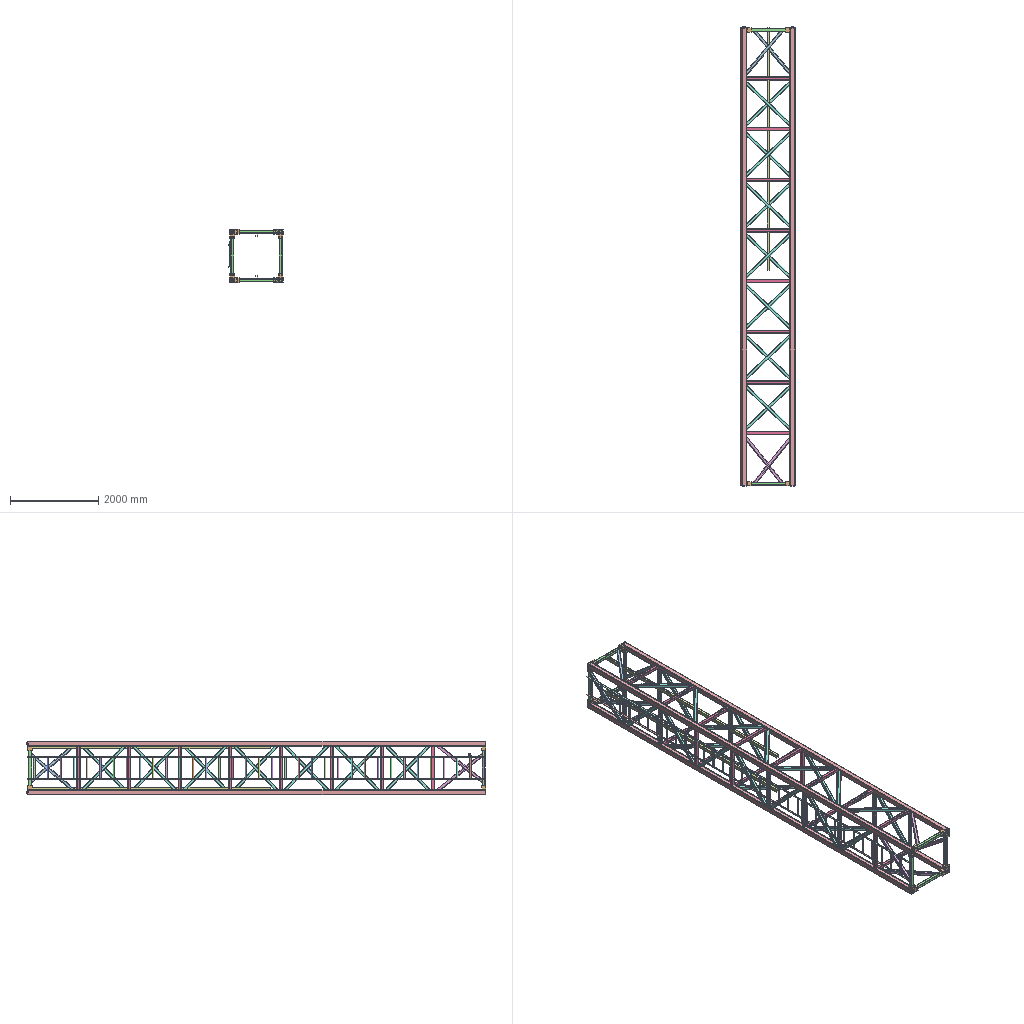Assembly | SolidWorks | 13 different items | 115 placed | box 1235 x 10440 x 1220 mm
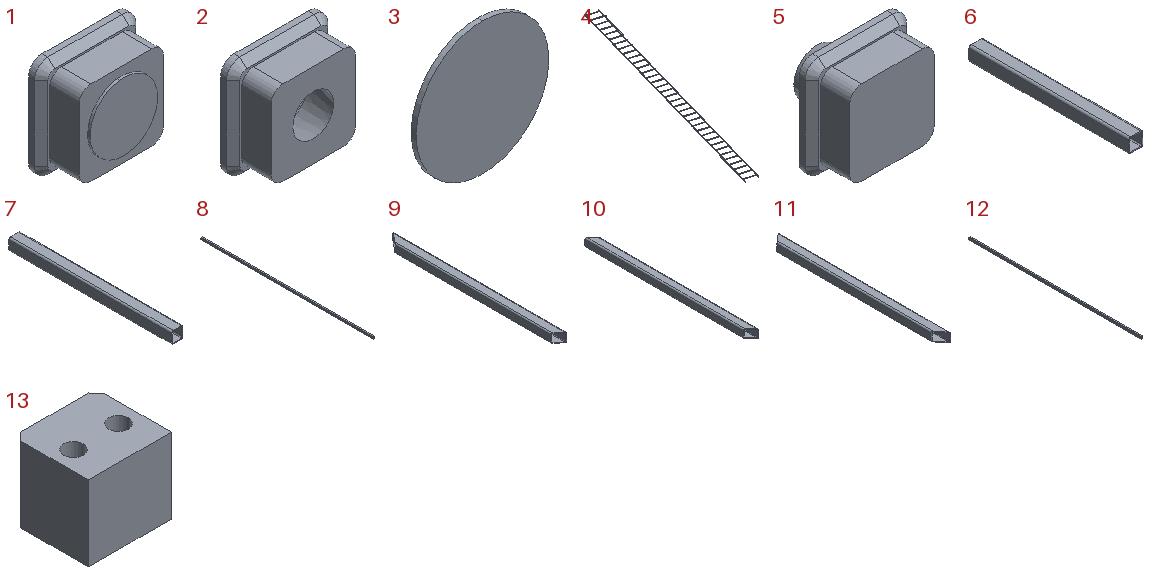Parts list (item | name | quantity | parent item | size | volume | features):
1 | (subassembly) | x4 | - | 120 x 53 x 120 mm | 407856 mm3 | -
2 | - | x4 | in 1 | 120 x 50 x 120 mm | 392776 mm3 | features Chamfer 1, Extrusion 1, ICE 1, RevCut 1
3 | - | x4 | in 1 | 80 x 3 x 80 mm | 15080 mm3 | features Extrusion 1
4 | - | x1 | - | 3347 x 10135 x 40 mm | 8856041 mm3 | features WeldMemberFeat 2, Chamfer 1, LPattern 1, Sweep 1, WeldCornerFeat 1, WeldmentFeature 1
5 | - | x4 | - | 120 x 90 x 120 mm | 672208 mm3 | features Chamfer 2, ICE 2, Revolution 1
6 | - | x8 | - | 70 x 780 x 70 mm | 963783 mm3 | features WeldMemberFeat 1, WeldmentFeature 1
7 | - | x32 | - | 70 x 980 x 70 mm | 1210907 mm3 | features WeldMemberFeat 1, WeldmentFeature 1
8 | - | x4 | - | 120 x 10370 x 120 mm | 43669629 mm3 | features WeldMemberFeat 1, WeldmentFeature 1
9 | - | x4 | - | 70 x 1340 x 70 mm | 1567074 mm3 | features ICE 1, WeldMemberFeat 1, WeldmentFeature 1
10 | - | x28 | - | 70 x 1421 x 70 mm | 1672765 mm3 | features ICE 1, WeldMemberFeat 1, WeldmentFeature 1
11 | - | x4 | - | 70 x 1302 x 70 mm | 1520953 mm3 | features ICE 1, WeldMemberFeat 1, WeldmentFeature 1
12 | - | x2 | - | 60 x 5500 x 80 mm | 6795907 mm3 | features WeldMemberFeat 1, WeldmentFeature 1
13 | - | x16 | - | 110 x 100 x 100 mm | 983814 mm3 | features Chamfer 1, Extrusion 1, HoleWzd 1
Mates (type | each side: item.copy, entity, surface, feature):
In the top assembly
Symmetric | 8.1 face plane Cold-formed Hollow Structural Square Steel(gb t6728-2002) 120×120×10(1) | 8.2 face plane Cold-formed Hollow Structural Square Steel(gb t6728-2002) 120×120×10(1) | assembly plane
DistanceDim | assembly plane | 8.1 face plane Cold-formed Hollow Structural Square Steel(gb t6728-2002) 120×120×10(1)
Coincident | 8.3 face plane Cold-formed Hollow Structural Square Steel(gb t6728-2002) 120×120×10(1) | assembly plane
Coincident | 8.1 face plane Cold-formed Hollow Structural Square Steel(gb t6728-2002) 120×120×10(1) | 2.1 face plane Boss-Extrude1
Width | 2.1 face plane Boss-Extrude2 | 2.1 face plane Boss-Extrude2 | 8.1 face plane Cold-formed Hollow Structural Square Steel(gb t6728-2002) 120×120×10(1) | 8.1 face plane Cold-formed Hollow Structural Square Steel(gb t6728-2002) 120×120×10(1)
Width | 8.1 face plane Cold-formed Hollow Structural Square Steel(gb t6728-2002) 120×120×10(1) | 8.1 face plane Cold-formed Hollow Structural Square Steel(gb t6728-2002) 120×120×10(1) | 2.1 face plane Boss-Extrude1 | 2.1 face plane Boss-Extrude1
Coincident | 8.1 face plane Cold-formed Hollow Structural Square Steel(gb t6728-2002) 120×120×10(1) | 5.1 face plane Boss-Extrude1
Width | 8.1 face plane Cold-formed Hollow Structural Square Steel(gb t6728-2002) 120×120×10(1) | 8.1 face plane Cold-formed Hollow Structural Square Steel(gb t6728-2002) 120×120×10(1) | 5.1 face plane Boss-Extrude1 | 5.1 face plane Boss-Extrude1 | 2 times
Coincident | 13.1 face plane Boss-Extrude1 | 2.2 face plane Boss-Extrude1
Width | 13.1 face plane Boss-Extrude1 | 13.1 face plane Boss-Extrude1 | 8.3 face plane Cold-formed Hollow Structural Square Steel(gb t6728-2002) 120×120×10(1) | 8.3 face plane Cold-formed Hollow Structural Square Steel(gb t6728-2002) 120×120×10(1)
Coincident | 13.1 face plane Boss-Extrude1 | 8.3 face plane Cold-formed Hollow Structural Square Steel(gb t6728-2002) 120×120×10(1)
Coincident | 8.3 face plane Cold-formed Hollow Structural Square Steel(gb t6728-2002) 120×120×10(1) | 13.2 face plane Boss-Extrude1
Coincident | 13.1 face plane Boss-Extrude1 | 13.2 face plane Boss-Extrude1
Width | 13.2 face plane Boss-Extrude1 | 13.2 face plane Boss-Extrude1 | 8.3 face plane Cold-formed Hollow Structural Square Steel(gb t6728-2002) 120×120×10(1) | 8.3 face plane Cold-formed Hollow Structural Square Steel(gb t6728-2002) 120×120×10(1)
Coincident | 13.3 face plane Boss-Extrude1 | 13.4 face plane Boss-Extrude1
Coincident | 13.1 face plane Boss-Extrude1 | 13.4 face plane Boss-Extrude1 | 2 times
Coincident | 13.2 face plane Boss-Extrude1 | 13.3 face plane Boss-Extrude1 | 2 times
Coincident | 5.2 face plane Boss-Extrude1 | 13.3 face plane Boss-Extrude1
Coincident | 6.1 face plane feature 19 (WeldMemberFeat) (+4 more in 5 files) Cold-formed Hollow Structural Square Steel(gb t6728-2002) 70×70×5(1) | 6.2 face plane feature 19 (WeldMemberFeat) (+4 more in 5 files) Cold-formed Hollow Structural Square Steel(gb t6728-2002) 70×70×5(1) | 2 times
Width | 6.2 face plane feature 19 (WeldMemberFeat) (+4 more in 5 files) Cold-formed Hollow Structural Square Steel(gb t6728-2002) 70×70×5(1) | 6.2 face plane feature 19 (WeldMemberFeat) (+4 more in 5 files) Cold-formed Hollow Structural Square Steel(gb t6728-2002) 70×70×5(1) | 13.5 face plane Boss-Extrude1 | 13.5 face plane Boss-Extrude1
Coincident | 13.1 face plane Boss-Extrude1 | 6.1 face plane feature 19 (WeldMemberFeat) (+4 more in 5 files) Cold-formed Hollow Structural Square Steel(gb t6728-2002) 70×70×5(1)
Width | 6.1 face plane feature 19 (WeldMemberFeat) (+4 more in 5 files) Cold-formed Hollow Structural Square Steel(gb t6728-2002) 70×70×5(1) | 6.1 face plane feature 19 (WeldMemberFeat) (+4 more in 5 files) Cold-formed Hollow Structural Square Steel(gb t6728-2002) 70×70×5(1) | 13.1 face plane Boss-Extrude1 | 13.1 face plane Boss-Extrude1
Width | 13.1 face plane Boss-Extrude1 | 13.1 face plane Boss-Extrude1 | 6.1 face plane feature 19 (WeldMemberFeat) (+4 more in 5 files) Cold-formed Hollow Structural Square Steel(gb t6728-2002) 70×70×5(1) | 6.1 face plane feature 19 (WeldMemberFeat) (+4 more in 5 files) Cold-formed Hollow Structural Square Steel(gb t6728-2002) 70×70×5(1)
Coincident | 6.3 face plane feature 19 (WeldMemberFeat) (+4 more in 5 files) Cold-formed Hollow Structural Square Steel(gb t6728-2002) 70×70×5(1) | 6.4 face plane feature 19 (WeldMemberFeat) (+4 more in 5 files) Cold-formed Hollow Structural Square Steel(gb t6728-2002) 70×70×5(1) | 2 times
Coincident | 13.2 face plane Boss-Extrude1 | 6.3 face plane feature 19 (WeldMemberFeat) (+4 more in 5 files) Cold-formed Hollow Structural Square Steel(gb t6728-2002) 70×70×5(1)
Width | 6.3 face plane feature 19 (WeldMemberFeat) (+4 more in 5 files) Cold-formed Hollow Structural Square Steel(gb t6728-2002) 70×70×5(1) | 6.3 face plane feature 19 (WeldMemberFeat) (+4 more in 5 files) Cold-formed Hollow Structural Square Steel(gb t6728-2002) 70×70×5(1) | 13.2 face plane Boss-Extrude1 | 13.2 face plane Boss-Extrude1 | 2 times
Width | 6.4 face plane feature 19 (WeldMemberFeat) (+4 more in 5 files) Cold-formed Hollow Structural Square Steel(gb t6728-2002) 70×70×5(1) | 6.4 face plane feature 19 (WeldMemberFeat) (+4 more in 5 files) Cold-formed Hollow Structural Square Steel(gb t6728-2002) 70×70×5(1) | 13.3 face plane Boss-Extrude1 | 13.3 face plane Boss-Extrude1
Width | 7.1 face plane feature 19 (WeldMemberFeat) (+4 more in 5 files) Cold-formed Hollow Structural Square Steel(gb t6728-2002) 70×70×5(1) | 7.1 face plane feature 19 (WeldMemberFeat) (+4 more in 5 files) Cold-formed Hollow Structural Square Steel(gb t6728-2002) 70×70×5(1) | 8.4 face plane Cold-formed Hollow Structural Square Steel(gb t6728-2002) 120×120×10(1) | 8.4 face plane Cold-formed Hollow Structural Square Steel(gb t6728-2002) 120×120×10(1)
Coincident | 7.1 face plane feature 19 (WeldMemberFeat) (+4 more in 5 files) Cold-formed Hollow Structural Square Steel(gb t6728-2002) 70×70×5(1) | 8.4 face plane Cold-formed Hollow Structural Square Steel(gb t6728-2002) 120×120×10(1)
DistanceDim | 2.2 face plane Boss-Extrude1 | 7.1 face plane feature 19 (WeldMemberFeat) (+4 more in 5 files) Cold-formed Hollow Structural Square Steel(gb t6728-2002) 70×70×5(1)
Coincident | 10.1 face plane Cut-Extrude1 | 8.4 face plane Cold-formed Hollow Structural Square Steel(gb t6728-2002) 120×120×10(1)
Coincident | 8.3 face plane Cold-formed Hollow Structural Square Steel(gb t6728-2002) 120×120×10(1) | 10.2 face plane Cut-Extrude1
Coincident | 10.1 face plane feature 19 (WeldMemberFeat) (+4 more in 5 files) Cold-formed Hollow Structural Square Steel(gb t6728-2002) 70×70×5(1) | 10.2 face plane feature 19 (WeldMemberFeat) (+4 more in 5 files) Cold-formed Hollow Structural Square Steel(gb t6728-2002) 70×70×5(1)
DistanceDim | 10.2 edge | 7.2 face plane feature 19 (WeldMemberFeat) (+4 more in 5 files) Cold-formed Hollow Structural Square Steel(gb t6728-2002) 70×70×5(1)
Coincident | 8.1 face plane Cold-formed Hollow Structural Square Steel(gb t6728-2002) 120×120×10(1) | 10.3 face plane Cut-Extrude1
Coincident | 7.3 face plane feature 19 (WeldMemberFeat) (+4 more in 5 files) Cold-formed Hollow Structural Square Steel(gb t6728-2002) 70×70×5(1) | 10.3 face plane feature 19 (WeldMemberFeat) (+4 more in 5 files) Cold-formed Hollow Structural Square Steel(gb t6728-2002) 70×70×5(1)
DistanceDim | 10.3 edge | 7.3 face plane feature 19 (WeldMemberFeat) (+4 more in 5 files) Cold-formed Hollow Structural Square Steel(gb t6728-2002) 70×70×5(1)
Coincident | 10.3 face plane feature 19 (WeldMemberFeat) (+4 more in 5 files) Cold-formed Hollow Structural Square Steel(gb t6728-2002) 70×70×5(1) | 10.4 face plane feature 19 (WeldMemberFeat) (+4 more in 5 files) Cold-formed Hollow Structural Square Steel(gb t6728-2002) 70×70×5(1)
Coincident | 8.2 face plane Cold-formed Hollow Structural Square Steel(gb t6728-2002) 120×120×10(1) | 10.4 face plane Cut-Extrude1
DistanceDim | 10.4 edge | 7.4 face plane feature 19 (WeldMemberFeat) (+4 more in 5 files) Cold-formed Hollow Structural Square Steel(gb t6728-2002) 70×70×5(1)
Coincident | 6.2 face plane feature 19 (WeldMemberFeat) (+4 more in 5 files) Cold-formed Hollow Structural Square Steel(gb t6728-2002) 70×70×5(1) | 11.1 face plane Cut-Extrude1
Coincident | 6.2 face plane feature 19 (WeldMemberFeat) (+4 more in 5 files) Cold-formed Hollow Structural Square Steel(gb t6728-2002) 70×70×5(1) | 11.1 face plane feature 19 (WeldMemberFeat) (+4 more in 5 files) Cold-formed Hollow Structural Square Steel(gb t6728-2002) 70×70×5(1)
Coincident | 8.3 face plane Cold-formed Hollow Structural Square Steel(gb t6728-2002) 120×120×10(1) | 11.1 face plane Cut-Extrude1
Coincident | 8.2 face plane Cold-formed Hollow Structural Square Steel(gb t6728-2002) 120×120×10(1) | 11.2 face plane Cut-Extrude1
Coincident | 7.5 face plane feature 19 (WeldMemberFeat) (+4 more in 5 files) Cold-formed Hollow Structural Square Steel(gb t6728-2002) 70×70×5(1) | 11.2 face plane feature 19 (WeldMemberFeat) (+4 more in 5 files) Cold-formed Hollow Structural Square Steel(gb t6728-2002) 70×70×5(1)
Coincident | 6.5 face plane feature 19 (WeldMemberFeat) (+4 more in 5 files) Cold-formed Hollow Structural Square Steel(gb t6728-2002) 70×70×5(1) | 11.2 face plane Cut-Extrude1
Coincident | 7.1 face plane feature 19 (WeldMemberFeat) (+4 more in 5 files) Cold-formed Hollow Structural Square Steel(gb t6728-2002) 70×70×5(1) | 7.6 face plane feature 19 (WeldMemberFeat) (+4 more in 5 files) Cold-formed Hollow Structural Square Steel(gb t6728-2002) 70×70×5(1)
Coincident | 8.3 face plane Cold-formed Hollow Structural Square Steel(gb t6728-2002) 120×120×10(1) | 7.6 face plane feature 19 (WeldMemberFeat) (+4 more in 5 files) Cold-formed Hollow Structural Square Steel(gb t6728-2002) 70×70×5(1)
Width | 7.6 face plane feature 19 (WeldMemberFeat) (+4 more in 5 files) Cold-formed Hollow Structural Square Steel(gb t6728-2002) 70×70×5(1) | 7.6 face plane feature 19 (WeldMemberFeat) (+4 more in 5 files) Cold-formed Hollow Structural Square Steel(gb t6728-2002) 70×70×5(1) | 8.3 face plane Cold-formed Hollow Structural Square Steel(gb t6728-2002) 120×120×10(1) | 8.3 face plane Cold-formed Hollow Structural Square Steel(gb t6728-2002) 120×120×10(1)
Coincident | 7.6 face plane feature 19 (WeldMemberFeat) (+4 more in 5 files) Cold-formed Hollow Structural Square Steel(gb t6728-2002) 70×70×5(1) | 7.7 face plane feature 19 (WeldMemberFeat) (+4 more in 5 files) Cold-formed Hollow Structural Square Steel(gb t6728-2002) 70×70×5(1) | 2 times
Width | 7.7 face plane feature 19 (WeldMemberFeat) (+4 more in 5 files) Cold-formed Hollow Structural Square Steel(gb t6728-2002) 70×70×5(1) | 7.7 face plane feature 19 (WeldMemberFeat) (+4 more in 5 files) Cold-formed Hollow Structural Square Steel(gb t6728-2002) 70×70×5(1) | 8.2 face plane Cold-formed Hollow Structural Square Steel(gb t6728-2002) 120×120×10(1) | 8.2 face plane Cold-formed Hollow Structural Square Steel(gb t6728-2002) 120×120×10(1)
Coincident | 4.1 face plane Gb/t 704—1988Hot-rolled Flat Steel 40×6(1) | 6.4 face plane feature 19 (WeldMemberFeat) (+4 more in 5 files) Cold-formed Hollow Structural Square Steel(gb t6728-2002) 70×70×5(1)
Width | 8.3 face plane Cold-formed Hollow Structural Square Steel(gb t6728-2002) 120×120×10(1) | 8.1 face plane Cold-formed Hollow Structural Square Steel(gb t6728-2002) 120×120×10(1) | 4.1 face plane Gb/t 704—1988Hot-rolled Flat Steel 40×6(1) | 4.1 face plane Gb/t 704—1988Hot-rolled Flat Steel 40×6(1)
Coincident | 4.1 face plane Gb/t 704—1988Hot-rolled Flat Steel 40×6(1) | 2.2 face plane Boss-Extrude1
Coincident | 6.2 face plane feature 19 (WeldMemberFeat) (+4 more in 5 files) Cold-formed Hollow Structural Square Steel(gb t6728-2002) 70×70×5(1) | 12.1 face plane Cold-formed Hollow Structural Rectangular Steel(gb t6728-2002) 80×60×5(1)
Coincident | 12.1 plane | assembly plane
Coincident | 12.1 face plane Cold-formed Hollow Structural Rectangular Steel(gb t6728-2002) 80×60×5(1) | 13.5 face plane Boss-Extrude1
Coincident | 9.1 face plane Cut-Extrude1 | 6.1 face plane feature 19 (WeldMemberFeat) (+4 more in 5 files) Cold-formed Hollow Structural Square Steel(gb t6728-2002) 70×70×5(1)
Coincident | 9.1 face plane feature 19 (WeldMemberFeat) (+4 more in 5 files) Cold-formed Hollow Structural Square Steel(gb t6728-2002) 70×70×5(1) | 6.1 face plane feature 19 (WeldMemberFeat) (+4 more in 5 files) Cold-formed Hollow Structural Square Steel(gb t6728-2002) 70×70×5(1)
Coincident | 9.1 face plane Cut-Extrude1 | 8.4 face plane Cold-formed Hollow Structural Square Steel(gb t6728-2002) 120×120×10(1)
Coincident | 6.6 face plane feature 19 (WeldMemberFeat) (+4 more in 5 files) Cold-formed Hollow Structural Square Steel(gb t6728-2002) 70×70×5(1) | 9.2 face plane Cut-Extrude1
Coincident | 6.6 face plane feature 19 (WeldMemberFeat) (+4 more in 5 files) Cold-formed Hollow Structural Square Steel(gb t6728-2002) 70×70×5(1) | 9.2 face plane feature 19 (WeldMemberFeat) (+4 more in 5 files) Cold-formed Hollow Structural Square Steel(gb t6728-2002) 70×70×5(1)
Coincident | 8.1 face plane Cold-formed Hollow Structural Square Steel(gb t6728-2002) 120×120×10(1) | 9.2 face plane Cut-Extrude1
Coincident | 6.3 face plane feature 19 (WeldMemberFeat) (+4 more in 5 files) Cold-formed Hollow Structural Square Steel(gb t6728-2002) 70×70×5(1) | 9.3 face plane Cut-Extrude1
Coincident | 6.3 face plane feature 19 (WeldMemberFeat) (+4 more in 5 files) Cold-formed Hollow Structural Square Steel(gb t6728-2002) 70×70×5(1) | 9.3 face plane feature 19 (WeldMemberFeat) (+4 more in 5 files) Cold-formed Hollow Structural Square Steel(gb t6728-2002) 70×70×5(1)
Coincident | 8.3 face plane Cold-formed Hollow Structural Square Steel(gb t6728-2002) 120×120×10(1) | 9.3 face plane Cut-Extrude1
Coincident | 6.7 face plane feature 19 (WeldMemberFeat) (+4 more in 5 files) Cold-formed Hollow Structural Square Steel(gb t6728-2002) 70×70×5(1) | 9.4 face plane Cut-Extrude1
Coincident | 6.7 face plane feature 19 (WeldMemberFeat) (+4 more in 5 files) Cold-formed Hollow Structural Square Steel(gb t6728-2002) 70×70×5(1) | 9.4 face plane feature 19 (WeldMemberFeat) (+4 more in 5 files) Cold-formed Hollow Structural Square Steel(gb t6728-2002) 70×70×5(1)
Coincident | 8.2 face plane Cold-formed Hollow Structural Square Steel(gb t6728-2002) 120×120×10(1) | 9.4 face plane Cut-Extrude1
Coincident | 8.1 face plane Cold-formed Hollow Structural Square Steel(gb t6728-2002) 120×120×10(1) | 11.3 face plane Cut-Extrude1
Coincident | 7.8 face plane feature 19 (WeldMemberFeat) (+4 more in 5 files) Cold-formed Hollow Structural Square Steel(gb t6728-2002) 70×70×5(1) | 11.3 face plane feature 19 (WeldMemberFeat) (+4 more in 5 files) Cold-formed Hollow Structural Square Steel(gb t6728-2002) 70×70×5(1)
Coincident | 6.4 face plane feature 19 (WeldMemberFeat) (+4 more in 5 files) Cold-formed Hollow Structural Square Steel(gb t6728-2002) 70×70×5(1) | 11.3 face plane Cut-Extrude1
Coincident | 6.8 face plane feature 19 (WeldMemberFeat) (+4 more in 5 files) Cold-formed Hollow Structural Square Steel(gb t6728-2002) 70×70×5(1) | 11.4 face plane Cut-Extrude1
Coincident | 7.9 face plane feature 19 (WeldMemberFeat) (+4 more in 5 files) Cold-formed Hollow Structural Square Steel(gb t6728-2002) 70×70×5(1) | 11.4 face plane feature 19 (WeldMemberFeat) (+4 more in 5 files) Cold-formed Hollow Structural Square Steel(gb t6728-2002) 70×70×5(1)
Coincident | 8.4 face plane Cold-formed Hollow Structural Square Steel(gb t6728-2002) 120×120×10(1) | 11.4 face plane Cut-Extrude1
Coincident | 8.1 face plane Cold-formed Hollow Structural Square Steel(gb t6728-2002) 120×120×10(1) | 10.5 face plane Cut-Extrude1
Coincident | 8.4 face plane Cold-formed Hollow Structural Square Steel(gb t6728-2002) 120×120×10(1) | 10.6 face plane Cut-Extrude1
Coincident | 7.7 face plane feature 19 (WeldMemberFeat) (+4 more in 5 files) Cold-formed Hollow Structural Square Steel(gb t6728-2002) 70×70×5(1) | 10.6 face plane feature 19 (WeldMemberFeat) (+4 more in 5 files) Cold-formed Hollow Structural Square Steel(gb t6728-2002) 70×70×5(1)
Coincident | 7.6 face plane feature 19 (WeldMemberFeat) (+4 more in 5 files) Cold-formed Hollow Structural Square Steel(gb t6728-2002) 70×70×5(1) | 10.5 face plane feature 19 (WeldMemberFeat) (+4 more in 5 files) Cold-formed Hollow Structural Square Steel(gb t6728-2002) 70×70×5(1)
DistanceDim | 10.5 edge | 7.6 face plane feature 19 (WeldMemberFeat) (+4 more in 5 files) Cold-formed Hollow Structural Square Steel(gb t6728-2002) 70×70×5(1)
DistanceDim | 10.6 edge | 7.7 face plane feature 19 (WeldMemberFeat) (+4 more in 5 files) Cold-formed Hollow Structural Square Steel(gb t6728-2002) 70×70×5(1)
Coincident | 8.3 face plane Cold-formed Hollow Structural Square Steel(gb t6728-2002) 120×120×10(1) | 10.7 face plane Cut-Extrude1
Coincident | 7.10 face plane feature 19 (WeldMemberFeat) (+4 more in 5 files) Cold-formed Hollow Structural Square Steel(gb t6728-2002) 70×70×5(1) | 10.7 face plane feature 19 (WeldMemberFeat) (+4 more in 5 files) Cold-formed Hollow Structural Square Steel(gb t6728-2002) 70×70×5(1)
DistanceDim | 7.10 face plane feature 19 (WeldMemberFeat) (+4 more in 5 files) Cold-formed Hollow Structural Square Steel(gb t6728-2002) 70×70×5(1) | 10.7 edge
Coincident | 8.4 face plane Cold-formed Hollow Structural Square Steel(gb t6728-2002) 120×120×10(1) | 10.8 face plane Cut-Extrude1
Coincident | 7.11 face plane feature 19 (WeldMemberFeat) (+4 more in 5 files) Cold-formed Hollow Structural Square Steel(gb t6728-2002) 70×70×5(1) | 10.8 face plane feature 19 (WeldMemberFeat) (+4 more in 5 files) Cold-formed Hollow Structural Square Steel(gb t6728-2002) 70×70×5(1)
DistanceDim | 7.11 face plane feature 19 (WeldMemberFeat) (+4 more in 5 files) Cold-formed Hollow Structural Square Steel(gb t6728-2002) 70×70×5(1) | 10.8 edge
DistanceDim | 10.1 edge | 7.1 face plane feature 19 (WeldMemberFeat) (+4 more in 5 files) Cold-formed Hollow Structural Square Steel(gb t6728-2002) 70×70×5(1)
Coincident | 10.1 face plane feature 19 (WeldMemberFeat) (+4 more in 5 files) Cold-formed Hollow Structural Square Steel(gb t6728-2002) 70×70×5(1) | 7.1 face plane feature 19 (WeldMemberFeat) (+4 more in 5 files) Cold-formed Hollow Structural Square Steel(gb t6728-2002) 70×70×5(1)
In subassembly 1
Concentric | 2.3 face cylinder Cut-Revolve1 | 3.1 face cylinder Boss-Extrude1
Coincident | 2.3 face plane Boss-Extrude2 | 3.1 face plane Boss-Extrude1